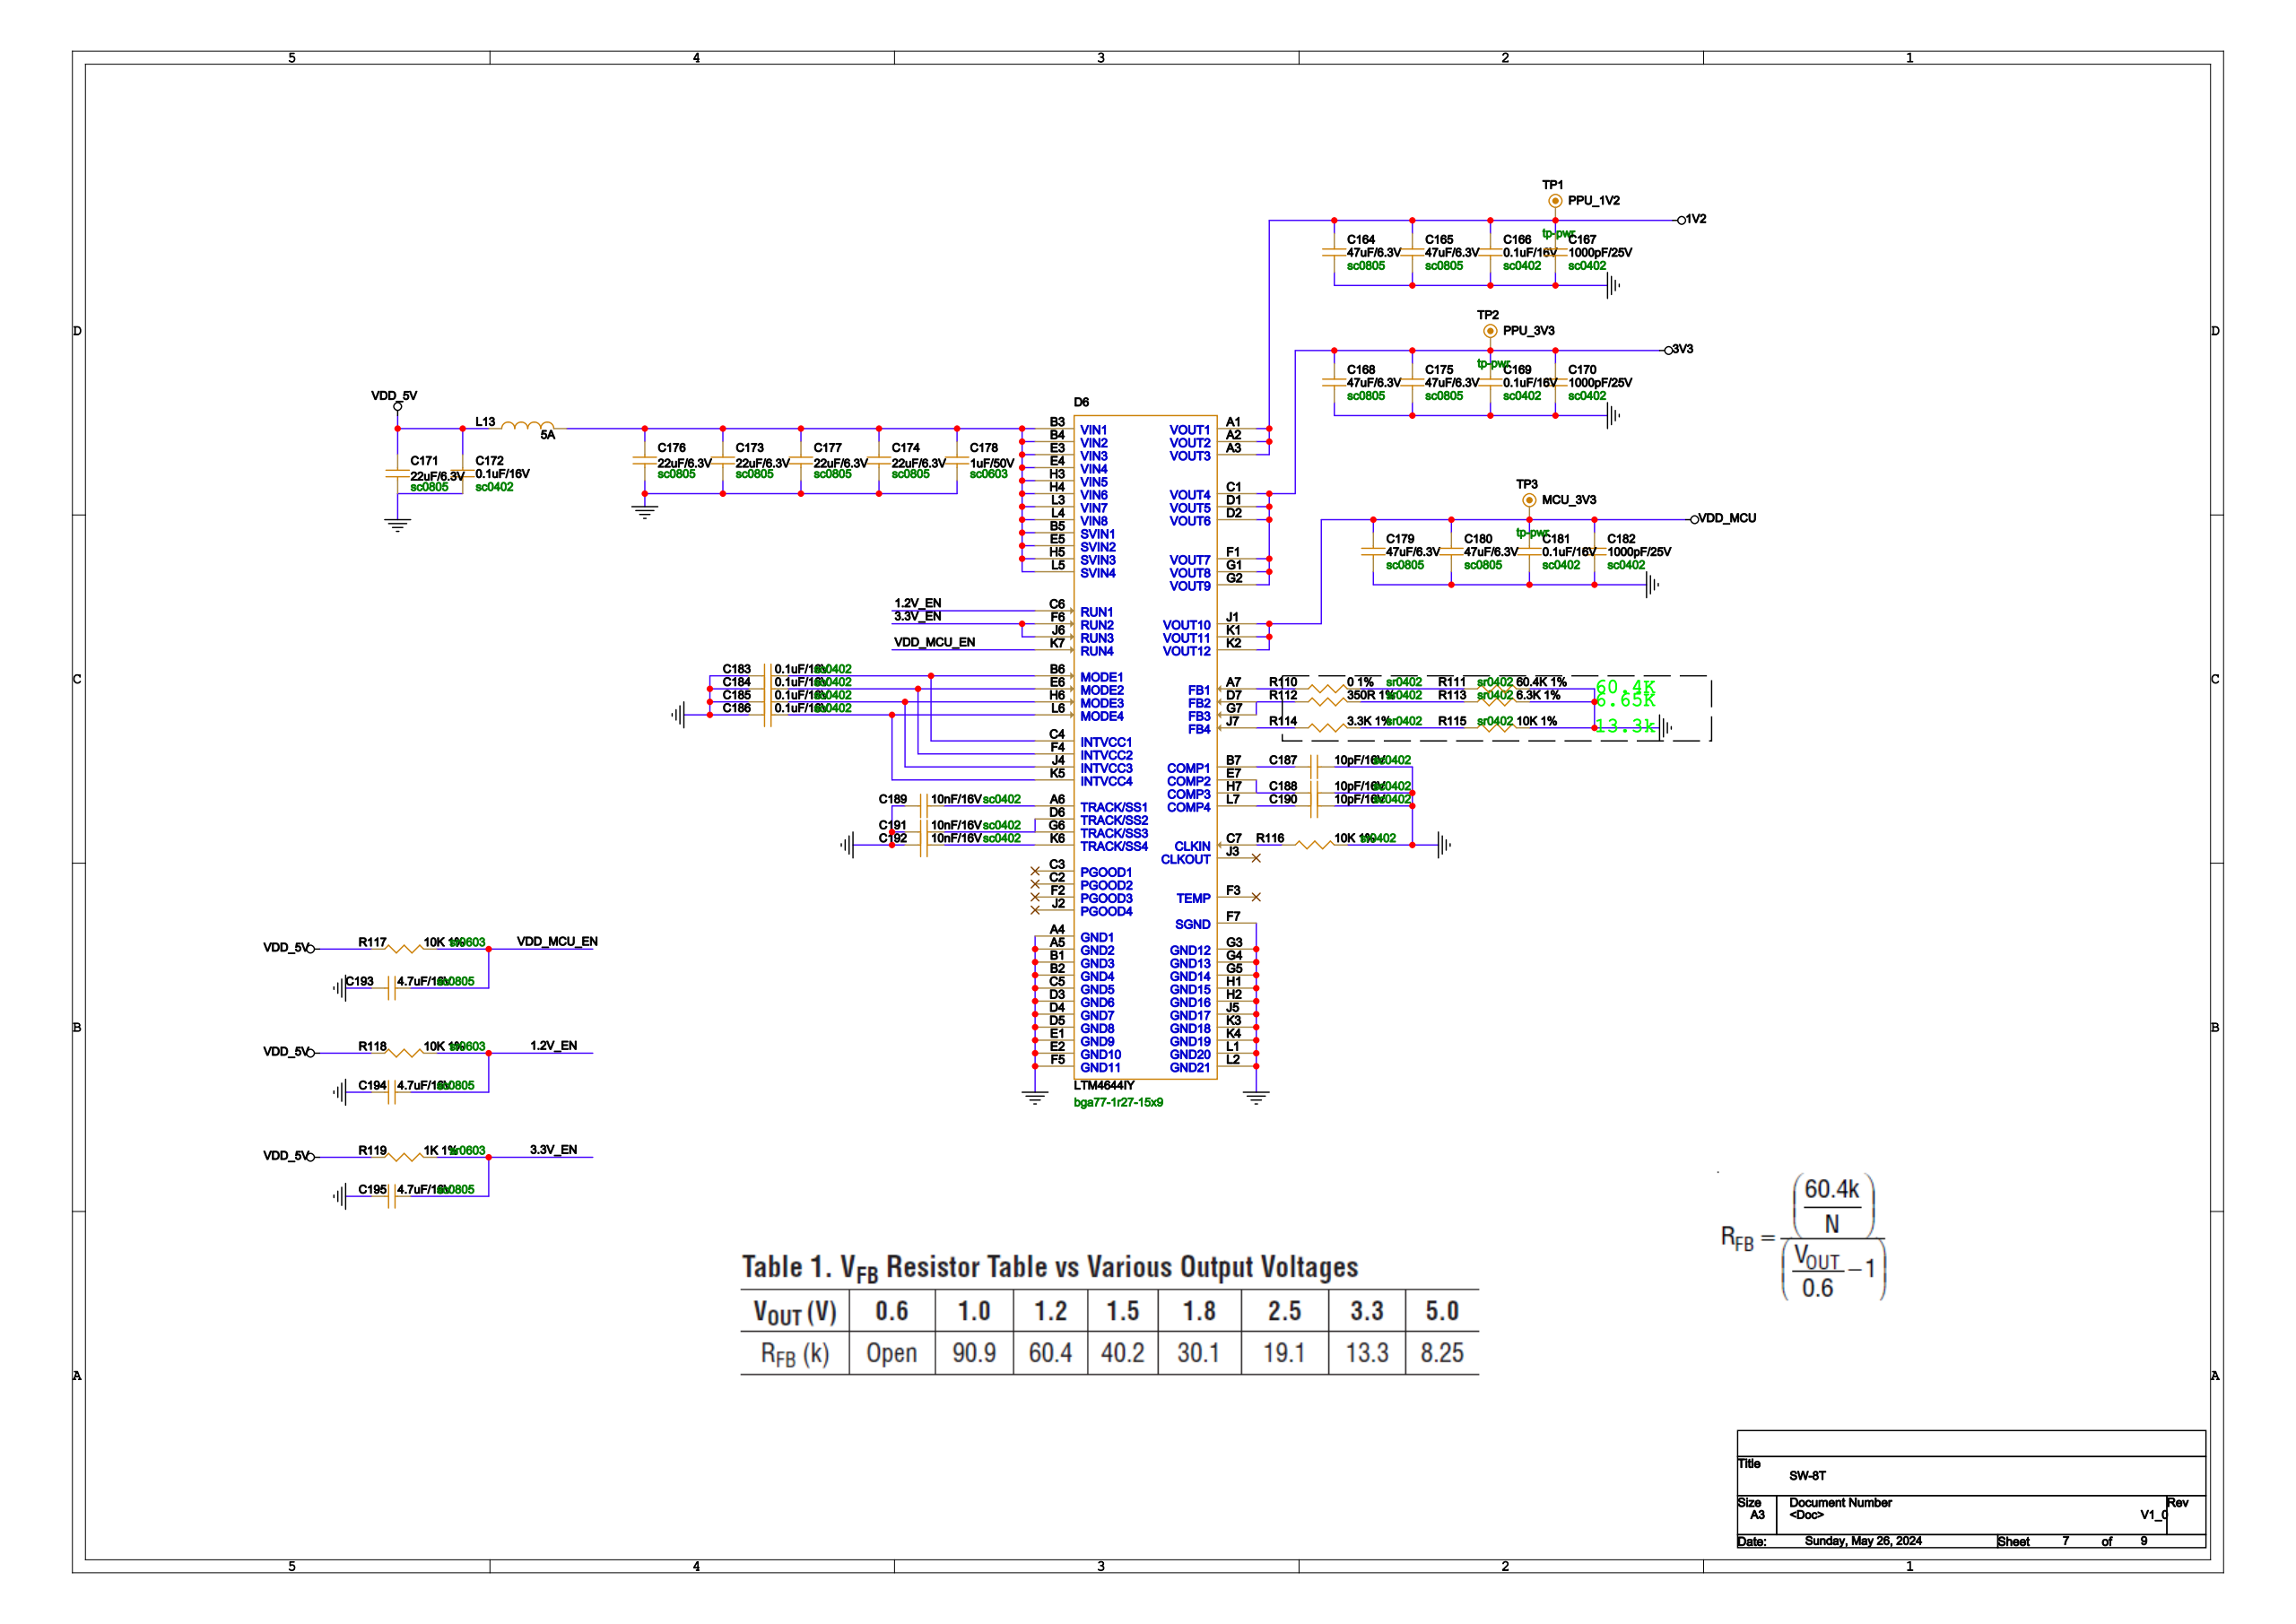Circuit board | Cadence Allegro | 399 parts | 387 nets | one sheet of the schematic
Parts on this sheet (reference | value | footprint):
C164 | 47uF/6.3V | SC0805
C165 | 47uF/6.3V | SC0805
C166 | 0.1uF/16V | SC0402
C167 | 1000pF/25V | SC0402
C168 | 47uF/6.3V | SC0805
C169 | 0.1uF/16V | SC0402
C170 | 1000pF/25V | SC0402
C171 | 22uF/6.3V | SC0805
C172 | 0.1uF/16V | SC0402
C173 | 22uF/6.3V | SC0805
C174 | 22uF/6.3V | SC0805
C175 | 47uF/6.3V | SC0805
C176 | 22uF/6.3V | SC0805
C177 | 22uF/6.3V | SC0805
C178 | 1uF/50V | SC0603
C179 | 47uF/6.3V | SC0805
C180 | 47uF/6.3V | SC0805
C181 | 0.1uF/16V | SC0402
C182 | 1000pF/25V | SC0402
C183 | 0.1uF/16V | SC0402
C184 | 0.1uF/16V | SC0402
C185 | 0.1uF/16V | SC0402
C186 | 0.1uF/16V | SC0402
C187 | 10pF/16V | SC0402
C188 | 10pF/16V | SC0402
C189 | 10nF/16V | SC0402
C190 | 10pF/16V | SC0402
C191 | 10nF/16V | SC0402
C192 | 10nF/16V | SC0402
C193 | 4.7uF/16V | SC0805
C194 | 4.7uF/16V | SC0805
C195 | 4.7uF/16V | SC0805
D6 | LTM4644IY | BGA77-1R27-15X9
L13 | 5A | SL0805
R110 | 0 1% | SR0402
R111 | 60.4K 1% | SR0402
R112 | 350R 1% | SR0402
R113 | 6.3K 1% | SR0402
R114 | 3.3K 1% | SR0402
R115 | 10K 1% | SR0402
R116 | 10K 1% | SR0402
R117 | 10K 1% | SR0603
R118 | 10K 1% | SR0603
R119 | 1K 1% | SR0603
TP1 | test_cir | TP-PWR
TP2 | test_cir | TP-PWR
TP3 | test_cir | TP-PWR
Nets of these parts (net: part-pin ...):
GND: C164-2 C165-2 C166-2 C167-2 C168-2 C169-2 C170-2 C171-2 C172-2 C173-2 C174-2 C175-2 C176-2 C177-2 C178-2 C179-2 C180-2 C181-2 C182-2 C183-1 C184-1 C185-1 C186-1 C187-2 C188-2 C189-1 C190-2 C191-1 C192-1 C193-2 C194-2 C195-2 R111-2 R113-2 R115-2 R116-2 D6-A4 D6-A5 D6-B1 D6-B2 D6-C5 D6-D3 D6-D4 D6-D5 D6-E1 D6-E2 D6-F5 D6-F7 D6-G3 D6-G4 D6-G5 D6-H1 D6-H2 D6-J5 D6-K3 D6-K4 D6-L1 D6-L2
VDD_MCU: C179-1 C180-1 C181-1 C182-1 TP3-1 D6-J1 D6-K1 D6-K2
3V3: C168-1 C169-1 C170-1 C175-1 TP2-1 D6-C1 D6-D1 D6-D2 D6-F1 D6-G1 D6-G2
VDD_5V: C171-1 C172-1 L13-1 R117-1 R118-1 R119-1
1V2: C164-1 C165-1 C166-1 C167-1 TP1-1 D6-A1 D6-A2 D6-A3
N17765268: C183-2 D6-B6 D6-C4
N17765266: C184-2 D6-E6 D6-F4
N17765276: C185-2 D6-H6 D6-J4
N17765280: C186-2 D6-K5 D6-L6
N17765517: C173-1 C174-1 C176-1 C177-1 C178-1 L13-2 D6-B3 D6-B4 D6-B5 D6-E3 D6-E4 D6-E5 D6-H3 D6-H4 D6-H5 D6-L3 D6-L4 D6-L5
N17765235: C187-1 D6-B7
N17765565: C188-1 D6-E7 D6-H7
N17765661: C190-1 D6-L7
N17764551: C189-2 D6-A6
N17765691: C191-2 D6-D6 D6-G6
N17765721: C192-2 D6-K6
VDD_MCU_EN: C193-1 R117-2 D6-K7
1.2V_EN: C194-1 R118-2 D6-C6
3.3V_EN: C195-1 R119-2 D6-F6 D6-J6
N17765677: R116-1 D6-C7
N17765860: R110-1 D6-A7
N17765252: R112-1 D6-D7 D6-G7
N17765549: R114-1 D6-J7
N17765222: R110-2 R111-1
N17765254: R112-2 R113-1
N17765551: R114-2 R115-1